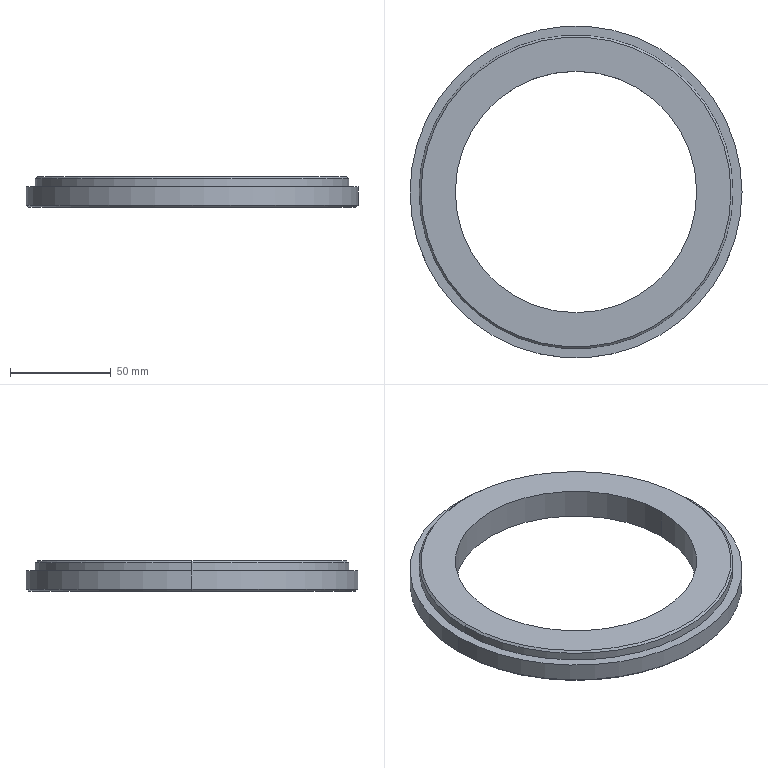Part | SolidWorks | features 3DProfileFeature 1, Chamfer 1, Extrusion 1, HoleWzd 1, ICE 1 | 1 solid | 37 faces | box 165 x 165 x 15 mm | volume 136481 mm3 | cylinder 18 | cone 16 | plane 3 | commonest cylinder face diameters 6.8 x12 120 x2 156 x2 165 x2
STEP:
#1=CARTESIAN_POINT('',(38.4,60.622,12.));
#2=VERTEX_POINT('',#1);
#3=CARTESIAN_POINT('',(31.6,60.622,12.));
#4=VERTEX_POINT('',#3);
#5=CARTESIAN_POINT('',(35.,60.622,12.));
#6=DIRECTION('',(0.,0.,-1.));
#7=DIRECTION('',(-1.,0.,0.));
#8=AXIS2_PLACEMENT_3D('',#5,#6,#7);
#9=CIRCLE('',#8,3.4);
#10=EDGE_CURVE('',#2,#4,#9,.T.);
#11=ORIENTED_EDGE('',*,*,#10,.F.);
#12=CARTESIAN_POINT('',(38.4,60.622,0.));
#13=VERTEX_POINT('',#12);
#14=CARTESIAN_POINT('',(38.4,60.622,0.));
#15=DIRECTION('',(0.,0.,-1.));
#16=VECTOR('',#15,1000.);
#17=LINE('',#14,#16);
#18=EDGE_CURVE('',#2,#13,#17,.T.);
#19=ORIENTED_EDGE('',*,*,#18,.T.);
#20=CARTESIAN_POINT('',(31.6,60.622,0.));
#21=VERTEX_POINT('',#20);
#22=CARTESIAN_POINT('',(35.,60.622,0.));
#23=DIRECTION('',(0.,0.,-1.));
#24=DIRECTION('',(-1.,0.,0.));
#25=AXIS2_PLACEMENT_3D('',#22,#23,#24);
#26=CIRCLE('',#25,3.4);
#27=EDGE_CURVE('',#13,#21,#26,.T.);
#28=ORIENTED_EDGE('',*,*,#27,.T.);
#29=CARTESIAN_POINT('',(31.6,60.622,0.));
#30=DIRECTION('',(0.,0.,-1.));
#31=VECTOR('',#30,1000.);
#32=LINE('',#29,#31);
#33=EDGE_CURVE('',#4,#21,#32,.T.);
#34=ORIENTED_EDGE('',*,*,#33,.F.);
#35=EDGE_LOOP('',(#11,#19,#28,#34));
#36=FACE_OUTER_BOUND('',#35,.T.);
#37=CARTESIAN_POINT('',(35.,60.622,0.));
#38=DIRECTION('',(0.,0.,-1.));
#39=DIRECTION('',(-1.,0.,0.));
#40=AXIS2_PLACEMENT_3D('',#37,#38,#39);
#41=CYLINDRICAL_SURFACE('',#40,3.4);
#42=ADVANCED_FACE('',(#36),#41,.F.);
#43=CARTESIAN_POINT('',(35.,60.622,14.043));
#44=VERTEX_POINT('',#43);
#45=CARTESIAN_POINT('',(31.6,60.622,12.));
#46=DIRECTION('',(-0.8572,0.,-0.515));
#47=VECTOR('',#46,1000.);
#48=LINE('',#45,#47);
#49=EDGE_CURVE('',#44,#4,#48,.T.);
#50=ORIENTED_EDGE('',*,*,#49,.F.);
#51=CARTESIAN_POINT('',(38.4,60.622,12.));
#52=DIRECTION('',(0.8572,0.,-0.515));
#53=VECTOR('',#52,1000.);
#54=LINE('',#51,#53);
#55=EDGE_CURVE('',#44,#2,#54,.T.);
#56=ORIENTED_EDGE('',*,*,#55,.T.);
#57=ORIENTED_EDGE('',*,*,#10,.T.);
#58=EDGE_LOOP('',(#50,#56,#57));
#59=FACE_OUTER_BOUND('',#58,.T.);
#60=CARTESIAN_POINT('',(35.,60.622,12.));
#61=DIRECTION('',(0.,0.,-1.));
#62=DIRECTION('',(-1.,0.,0.));
#63=AXIS2_PLACEMENT_3D('',#60,#61,#62);
#64=CONICAL_SURFACE('',#63,3.4,1.03);
#65=ADVANCED_FACE('',(#59),#64,.F.);
#66=CARTESIAN_POINT('',(-31.6,60.622,12.));
#67=VERTEX_POINT('',#66);
#68=CARTESIAN_POINT('',(-38.4,60.622,12.));
#69=VERTEX_POINT('',#68);
#70=CARTESIAN_POINT('',(-35.,60.622,12.));
#71=DIRECTION('',(0.,0.,-1.));
#72=DIRECTION('',(-1.,0.,0.));
#73=AXIS2_PLACEMENT_3D('',#70,#71,#72);
#74=CIRCLE('',#73,3.4);
#75=EDGE_CURVE('',#67,#69,#74,.T.);
#76=ORIENTED_EDGE('',*,*,#75,.F.);
#77=CARTESIAN_POINT('',(-31.6,60.622,0.));
#78=VERTEX_POINT('',#77);
#79=CARTESIAN_POINT('',(-31.6,60.622,0.));
#80=DIRECTION('',(0.,0.,-1.));
#81=VECTOR('',#80,1000.);
#82=LINE('',#79,#81);
#83=EDGE_CURVE('',#67,#78,#82,.T.);
#84=ORIENTED_EDGE('',*,*,#83,.T.);
#85=CARTESIAN_POINT('',(-38.4,60.622,0.));
#86=VERTEX_POINT('',#85);
#87=CARTESIAN_POINT('',(-35.,60.622,0.));
#88=DIRECTION('',(0.,0.,-1.));
#89=DIRECTION('',(-1.,0.,0.));
#90=AXIS2_PLACEMENT_3D('',#87,#88,#89);
#91=CIRCLE('',#90,3.4);
#92=EDGE_CURVE('',#78,#86,#91,.T.);
#93=ORIENTED_EDGE('',*,*,#92,.T.);
#94=CARTESIAN_POINT('',(-38.4,60.622,0.));
#95=DIRECTION('',(0.,0.,-1.));
#96=VECTOR('',#95,1000.);
#97=LINE('',#94,#96);
#98=EDGE_CURVE('',#69,#86,#97,.T.);
#99=ORIENTED_EDGE('',*,*,#98,.F.);
#100=EDGE_LOOP('',(#76,#84,#93,#99));
#101=FACE_OUTER_BOUND('',#100,.T.);
#102=CARTESIAN_POINT('',(-35.,60.622,0.));
#103=DIRECTION('',(0.,0.,-1.));
#104=DIRECTION('',(-1.,0.,0.));
#105=AXIS2_PLACEMENT_3D('',#102,#103,#104);
#106=CYLINDRICAL_SURFACE('',#105,3.4);
#107=ADVANCED_FACE('',(#101),#106,.F.);
#108=CARTESIAN_POINT('',(-35.,60.622,14.043));
#109=VERTEX_POINT('',#108);
#110=CARTESIAN_POINT('',(-38.4,60.622,12.));
#111=DIRECTION('',(-0.8572,0.,-0.515));
#112=VECTOR('',#111,1000.);
#113=LINE('',#110,#112);
#114=EDGE_CURVE('',#109,#69,#113,.T.);
#115=ORIENTED_EDGE('',*,*,#114,.F.);
#116=CARTESIAN_POINT('',(-31.6,60.622,12.));
#117=DIRECTION('',(0.8572,0.,-0.515));
#118=VECTOR('',#117,1000.);
#119=LINE('',#116,#118);
#120=EDGE_CURVE('',#109,#67,#119,.T.);
#121=ORIENTED_EDGE('',*,*,#120,.T.);
#122=ORIENTED_EDGE('',*,*,#75,.T.);
#123=EDGE_LOOP('',(#115,#121,#122));
#124=FACE_OUTER_BOUND('',#123,.T.);
#125=CARTESIAN_POINT('',(-35.,60.622,12.));
#126=DIRECTION('',(0.,0.,-1.));
#127=DIRECTION('',(-1.,0.,0.));
#128=AXIS2_PLACEMENT_3D('',#125,#126,#127);
#129=CONICAL_SURFACE('',#128,3.4,1.03);
#130=ADVANCED_FACE('',(#124),#129,.F.);
#131=CARTESIAN_POINT('',(-66.6,0.,12.));
#132=VERTEX_POINT('',#131);
#133=CARTESIAN_POINT('',(-73.4,0.,12.));
#134=VERTEX_POINT('',#133);
#135=CARTESIAN_POINT('',(-70.,0.,12.));
#136=DIRECTION('',(0.,0.,-1.));
#137=DIRECTION('',(-1.,0.,0.));
#138=AXIS2_PLACEMENT_3D('',#135,#136,#137);
#139=CIRCLE('',#138,3.4);
#140=EDGE_CURVE('',#132,#134,#139,.T.);
#141=ORIENTED_EDGE('',*,*,#140,.F.);
#142=CARTESIAN_POINT('',(-66.6,0.,0.));
#143=VERTEX_POINT('',#142);
#144=CARTESIAN_POINT('',(-66.6,0.,0.));
#145=DIRECTION('',(0.,0.,-1.));
#146=VECTOR('',#145,1000.);
#147=LINE('',#144,#146);
#148=EDGE_CURVE('',#132,#143,#147,.T.);
#149=ORIENTED_EDGE('',*,*,#148,.T.);
#150=CARTESIAN_POINT('',(-73.4,0.,0.));
#151=VERTEX_POINT('',#150);
#152=CARTESIAN_POINT('',(-70.,0.,0.));
#153=DIRECTION('',(0.,0.,-1.));
#154=DIRECTION('',(-1.,0.,0.));
#155=AXIS2_PLACEMENT_3D('',#152,#153,#154);
#156=CIRCLE('',#155,3.4);
#157=EDGE_CURVE('',#143,#151,#156,.T.);
#158=ORIENTED_EDGE('',*,*,#157,.T.);
#159=CARTESIAN_POINT('',(-73.4,0.,0.));
#160=DIRECTION('',(0.,0.,-1.));
#161=VECTOR('',#160,1000.);
#162=LINE('',#159,#161);
#163=EDGE_CURVE('',#134,#151,#162,.T.);
#164=ORIENTED_EDGE('',*,*,#163,.F.);
#165=EDGE_LOOP('',(#141,#149,#158,#164));
#166=FACE_OUTER_BOUND('',#165,.T.);
#167=CARTESIAN_POINT('',(-70.,0.,0.));
#168=DIRECTION('',(0.,0.,-1.));
#169=DIRECTION('',(-1.,0.,0.));
#170=AXIS2_PLACEMENT_3D('',#167,#168,#169);
#171=CYLINDRICAL_SURFACE('',#170,3.4);
#172=ADVANCED_FACE('',(#166),#171,.F.);
#173=CARTESIAN_POINT('',(-70.,0.,14.043));
#174=VERTEX_POINT('',#173);
#175=CARTESIAN_POINT('',(-73.4,0.,12.));
#176=DIRECTION('',(-0.8572,0.,-0.515));
#177=VECTOR('',#176,1000.);
#178=LINE('',#175,#177);
#179=EDGE_CURVE('',#174,#134,#178,.T.);
#180=ORIENTED_EDGE('',*,*,#179,.F.);
#181=CARTESIAN_POINT('',(-66.6,0.,12.));
#182=DIRECTION('',(0.8572,0.,-0.515));
#183=VECTOR('',#182,1000.);
#184=LINE('',#181,#183);
#185=EDGE_CURVE('',#174,#132,#184,.T.);
#186=ORIENTED_EDGE('',*,*,#185,.T.);
#187=ORIENTED_EDGE('',*,*,#140,.T.);
#188=EDGE_LOOP('',(#180,#186,#187));
#189=FACE_OUTER_BOUND('',#188,.T.);
#190=CARTESIAN_POINT('',(-70.,0.,12.));
#191=DIRECTION('',(0.,0.,-1.));
#192=DIRECTION('',(-1.,0.,0.));
#193=AXIS2_PLACEMENT_3D('',#190,#191,#192);
#194=CONICAL_SURFACE('',#193,3.4,1.03);
#195=ADVANCED_FACE('',(#189),#194,.F.);
#196=CARTESIAN_POINT('',(-31.6,-60.622,12.));
#197=VERTEX_POINT('',#196);
#198=CARTESIAN_POINT('',(-38.4,-60.622,12.));
#199=VERTEX_POINT('',#198);
#200=CARTESIAN_POINT('',(-35.,-60.622,12.));
#201=DIRECTION('',(0.,0.,-1.));
#202=DIRECTION('',(-1.,0.,0.));
#203=AXIS2_PLACEMENT_3D('',#200,#201,#202);
#204=CIRCLE('',#203,3.4);
#205=EDGE_CURVE('',#197,#199,#204,.T.);
#206=ORIENTED_EDGE('',*,*,#205,.F.);
#207=CARTESIAN_POINT('',(-31.6,-60.622,0.));
#208=VERTEX_POINT('',#207);
#209=CARTESIAN_POINT('',(-31.6,-60.622,0.));
#210=DIRECTION('',(0.,0.,-1.));
#211=VECTOR('',#210,1000.);
#212=LINE('',#209,#211);
#213=EDGE_CURVE('',#197,#208,#212,.T.);
#214=ORIENTED_EDGE('',*,*,#213,.T.);
#215=CARTESIAN_POINT('',(-38.4,-60.622,0.));
#216=VERTEX_POINT('',#215);
#217=CARTESIAN_POINT('',(-35.,-60.622,0.));
#218=DIRECTION('',(0.,0.,-1.));
#219=DIRECTION('',(-1.,0.,0.));
#220=AXIS2_PLACEMENT_3D('',#217,#218,#219);
#221=CIRCLE('',#220,3.4);
#222=EDGE_CURVE('',#208,#216,#221,.T.);
#223=ORIENTED_EDGE('',*,*,#222,.T.);
#224=CARTESIAN_POINT('',(-38.4,-60.622,0.));
#225=DIRECTION('',(0.,0.,-1.));
#226=VECTOR('',#225,1000.);
#227=LINE('',#224,#226);
#228=EDGE_CURVE('',#199,#216,#227,.T.);
#229=ORIENTED_EDGE('',*,*,#228,.F.);
#230=EDGE_LOOP('',(#206,#214,#223,#229));
#231=FACE_OUTER_BOUND('',#230,.T.);
#232=CARTESIAN_POINT('',(-35.,-60.622,0.));
#233=DIRECTION('',(0.,0.,-1.));
#234=DIRECTION('',(-1.,0.,0.));
#235=AXIS2_PLACEMENT_3D('',#232,#233,#234);
#236=CYLINDRICAL_SURFACE('',#235,3.4);
#237=ADVANCED_FACE('',(#231),#236,.F.);
#238=CARTESIAN_POINT('',(-35.,-60.622,14.043));
#239=VERTEX_POINT('',#238);
#240=CARTESIAN_POINT('',(-38.4,-60.622,12.));
#241=DIRECTION('',(-0.8572,0.,-0.515));
#242=VECTOR('',#241,1000.);
#243=LINE('',#240,#242);
#244=EDGE_CURVE('',#239,#199,#243,.T.);
#245=ORIENTED_EDGE('',*,*,#244,.F.);
#246=CARTESIAN_POINT('',(-31.6,-60.622,12.));
#247=DIRECTION('',(0.8572,0.,-0.515));
#248=VECTOR('',#247,1000.);
#249=LINE('',#246,#248);
#250=EDGE_CURVE('',#239,#197,#249,.T.);
#251=ORIENTED_EDGE('',*,*,#250,.T.);
#252=ORIENTED_EDGE('',*,*,#205,.T.);
#253=EDGE_LOOP('',(#245,#251,#252));
#254=FACE_OUTER_BOUND('',#253,.T.);
#255=CARTESIAN_POINT('',(-35.,-60.622,12.));
#256=DIRECTION('',(0.,0.,-1.));
#257=DIRECTION('',(-1.,0.,0.));
#258=AXIS2_PLACEMENT_3D('',#255,#256,#257);
#259=CONICAL_SURFACE('',#258,3.4,1.03);
#260=ADVANCED_FACE('',(#254),#259,.F.);
#261=CARTESIAN_POINT('',(38.4,-60.622,12.));
#262=VERTEX_POINT('',#261);
#263=CARTESIAN_POINT('',(31.6,-60.622,12.));
#264=VERTEX_POINT('',#263);
#265=CARTESIAN_POINT('',(35.,-60.622,12.));
#266=DIRECTION('',(0.,0.,-1.));
#267=DIRECTION('',(-1.,0.,0.));
#268=AXIS2_PLACEMENT_3D('',#265,#266,#267);
#269=CIRCLE('',#268,3.4);
#270=EDGE_CURVE('',#262,#264,#269,.T.);
#271=ORIENTED_EDGE('',*,*,#270,.F.);
#272=CARTESIAN_POINT('',(38.4,-60.622,0.));
#273=VERTEX_POINT('',#272);
#274=CARTESIAN_POINT('',(38.4,-60.622,0.));
#275=DIRECTION('',(0.,0.,-1.));
#276=VECTOR('',#275,1000.);
#277=LINE('',#274,#276);
#278=EDGE_CURVE('',#262,#273,#277,.T.);
#279=ORIENTED_EDGE('',*,*,#278,.T.);
#280=CARTESIAN_POINT('',(31.6,-60.622,0.));
#281=VERTEX_POINT('',#280);
#282=CARTESIAN_POINT('',(35.,-60.622,0.));
#283=DIRECTION('',(0.,0.,-1.));
#284=DIRECTION('',(-1.,0.,0.));
#285=AXIS2_PLACEMENT_3D('',#282,#283,#284);
#286=CIRCLE('',#285,3.4);
#287=EDGE_CURVE('',#273,#281,#286,.T.);
#288=ORIENTED_EDGE('',*,*,#287,.T.);
#289=CARTESIAN_POINT('',(31.6,-60.622,0.));
#290=DIRECTION('',(0.,0.,-1.));
#291=VECTOR('',#290,1000.);
#292=LINE('',#289,#291);
#293=EDGE_CURVE('',#264,#281,#292,.T.);
#294=ORIENTED_EDGE('',*,*,#293,.F.);
#295=EDGE_LOOP('',(#271,#279,#288,#294));
#296=FACE_OUTER_BOUND('',#295,.T.);
#297=CARTESIAN_POINT('',(35.,-60.622,0.));
#298=DIRECTION('',(0.,0.,-1.));
#299=DIRECTION('',(-1.,0.,0.));
#300=AXIS2_PLACEMENT_3D('',#297,#298,#299);
#301=CYLINDRICAL_SURFACE('',#300,3.4);
#302=ADVANCED_FACE('',(#296),#301,.F.);
#303=CARTESIAN_POINT('',(35.,-60.622,14.043));
#304=VERTEX_POINT('',#303);
#305=CARTESIAN_POINT('',(31.6,-60.622,12.));
#306=DIRECTION('',(-0.8572,0.,-0.515));
#307=VECTOR('',#306,1000.);
#308=LINE('',#305,#307);
#309=EDGE_CURVE('',#304,#264,#308,.T.);
#310=ORIENTED_EDGE('',*,*,#309,.F.);
#311=CARTESIAN_POINT('',(38.4,-60.622,12.));
#312=DIRECTION('',(0.8572,0.,-0.515));
#313=VECTOR('',#312,1000.);
#314=LINE('',#311,#313);
#315=EDGE_CURVE('',#304,#262,#314,.T.);
#316=ORIENTED_EDGE('',*,*,#315,.T.);
#317=ORIENTED_EDGE('',*,*,#270,.T.);
#318=EDGE_LOOP('',(#310,#316,#317));
#319=FACE_OUTER_BOUND('',#318,.T.);
#320=CARTESIAN_POINT('',(35.,-60.622,12.));
#321=DIRECTION('',(0.,0.,-1.));
#322=DIRECTION('',(-1.,0.,0.));
#323=AXIS2_PLACEMENT_3D('',#320,#321,#322);
#324=CONICAL_SURFACE('',#323,3.4,1.03);
#325=ADVANCED_FACE('',(#319),#324,.F.);
#326=CARTESIAN_POINT('',(73.4,0.,12.));
#327=VERTEX_POINT('',#326);
#328=CARTESIAN_POINT('',(66.6,0.,12.));
#329=VERTEX_POINT('',#328);
#330=CARTESIAN_POINT('',(70.,0.,12.));
#331=DIRECTION('',(0.,0.,-1.));
#332=DIRECTION('',(-1.,0.,0.));
#333=AXIS2_PLACEMENT_3D('',#330,#331,#332);
#334=CIRCLE('',#333,3.4);
#335=EDGE_CURVE('',#327,#329,#334,.T.);
#336=ORIENTED_EDGE('',*,*,#335,.F.);
#337=CARTESIAN_POINT('',(73.4,0.,0.));
#338=VERTEX_POINT('',#337);
#339=CARTESIAN_POINT('',(73.4,0.,0.));
#340=DIRECTION('',(0.,0.,-1.));
#341=VECTOR('',#340,1000.);
#342=LINE('',#339,#341);
#343=EDGE_CURVE('',#327,#338,#342,.T.);
#344=ORIENTED_EDGE('',*,*,#343,.T.);
#345=CARTESIAN_POINT('',(66.6,0.,0.));
#346=VERTEX_POINT('',#345);
#347=CARTESIAN_POINT('',(70.,0.,0.));
#348=DIRECTION('',(0.,0.,-1.));
#349=DIRECTION('',(-1.,0.,0.));
#350=AXIS2_PLACEMENT_3D('',#347,#348,#349);
#351=CIRCLE('',#350,3.4);
#352=EDGE_CURVE('',#338,#346,#351,.T.);
#353=ORIENTED_EDGE('',*,*,#352,.T.);
#354=CARTESIAN_POINT('',(66.6,0.,0.));
#355=DIRECTION('',(0.,0.,-1.));
#356=VECTOR('',#355,1000.);
#357=LINE('',#354,#356);
#358=EDGE_CURVE('',#329,#346,#357,.T.);
#359=ORIENTED_EDGE('',*,*,#358,.F.);
#360=EDGE_LOOP('',(#336,#344,#353,#359));
#361=FACE_OUTER_BOUND('',#360,.T.);
#362=CARTESIAN_POINT('',(70.,0.,0.));
#363=DIRECTION('',(0.,0.,-1.));
#364=DIRECTION('',(-1.,0.,0.));
#365=AXIS2_PLACEMENT_3D('',#362,#363,#364);
#366=CYLINDRICAL_SURFACE('',#365,3.4);
#367=ADVANCED_FACE('',(#361),#366,.F.);
#368=CARTESIAN_POINT('',(70.,0.,14.043));
#369=VERTEX_POINT('',#368);
#370=CARTESIAN_POINT('',(66.6,0.,12.));
#371=DIRECTION('',(-0.8572,0.,-0.515));
#372=VECTOR('',#371,1000.);
#373=LINE('',#370,#372);
#374=EDGE_CURVE('',#369,#329,#373,.T.);
#375=ORIENTED_EDGE('',*,*,#374,.F.);
#376=CARTESIAN_POINT('',(73.4,0.,12.));
#377=DIRECTION('',(0.8572,0.,-0.515));
#378=VECTOR('',#377,1000.);
#379=LINE('',#376,#378);
#380=EDGE_CURVE('',#369,#327,#379,.T.);
#381=ORIENTED_EDGE('',*,*,#380,.T.);
#382=ORIENTED_EDGE('',*,*,#335,.T.);
#383=EDGE_LOOP('',(#375,#381,#382));
#384=FACE_OUTER_BOUND('',#383,.T.);
#385=CARTESIAN_POINT('',(70.,0.,12.));
#386=DIRECTION('',(0.,0.,-1.));
#387=DIRECTION('',(-1.,0.,0.));
#388=AXIS2_PLACEMENT_3D('',#385,#386,#387);
#389=CONICAL_SURFACE('',#388,3.4,1.03);
#390=ADVANCED_FACE('',(#384),#389,.F.);
#391=CARTESIAN_POINT('',(77.,0.,15.));
#392=VERTEX_POINT('',#391);
#393=CARTESIAN_POINT('',(-77.,0.,15.));
#394=VERTEX_POINT('',#393);
#395=CARTESIAN_POINT('',(0.,0.,15.));
#396=DIRECTION('',(0.,0.,1.));
#397=DIRECTION('',(1.,0.,0.));
#398=AXIS2_PLACEMENT_3D('',#395,#396,#397);
#399=CIRCLE('',#398,77.);
#400=EDGE_CURVE('',#392,#394,#399,.T.);
#401=ORIENTED_EDGE('',*,*,#400,.F.);
#402=CARTESIAN_POINT('',(78.,0.,14.));
#403=VERTEX_POINT('',#402);
#404=CARTESIAN_POINT('',(77.,0.,15.));
#405=DIRECTION('',(0.7071,0.,-0.7071));
#406=VECTOR('',#405,1000.);
#407=LINE('',#404,#406);
#408=EDGE_CURVE('',#392,#403,#407,.T.);
#409=ORIENTED_EDGE('',*,*,#408,.T.);
#410=CARTESIAN_POINT('',(-78.,0.,14.));
#411=VERTEX_POINT('',#410);
#412=CARTESIAN_POINT('',(0.,0.,14.));
#413=DIRECTION('',(0.,0.,-1.));
#414=DIRECTION('',(1.,0.,0.));
#415=AXIS2_PLACEMENT_3D('',#412,#413,#414);
#416=CIRCLE('',#415,78.);
#417=EDGE_CURVE('',#411,#403,#416,.T.);
#418=ORIENTED_EDGE('',*,*,#417,.F.);
#419=CARTESIAN_POINT('',(-77.,0.,15.));
#420=DIRECTION('',(-0.7071,0.,-0.7071));
#421=VECTOR('',#420,1000.);
#422=LINE('',#419,#421);
#423=EDGE_CURVE('',#394,#411,#422,.T.);
#424=ORIENTED_EDGE('',*,*,#423,.F.);
#425=EDGE_LOOP('',(#401,#409,#418,#424));
#426=FACE_OUTER_BOUND('',#425,.T.);
#427=CARTESIAN_POINT('',(0.,0.,15.));
#428=DIRECTION('',(0.,0.,-1.));
#429=DIRECTION('',(-1.,0.,0.));
#430=AXIS2_PLACEMENT_3D('',#427,#428,#429);
#431=CONICAL_SURFACE('',#430,77.,0.7854);
#432=ADVANCED_FACE('',(#426),#431,.T.);
#433=CARTESIAN_POINT('',(-81.5,0.,0.));
#434=VERTEX_POINT('',#433);
#435=CARTESIAN_POINT('',(81.5,0.,0.));
#436=VERTEX_POINT('',#435);
#437=CARTESIAN_POINT('',(0.,0.,0.));
#438=DIRECTION('',(0.,0.,-1.));
#439=DIRECTION('',(1.,0.,0.));
#440=AXIS2_PLACEMENT_3D('',#437,#438,#439);
#441=CIRCLE('',#440,81.5);
#442=EDGE_CURVE('',#434,#436,#441,.T.);
#443=ORIENTED_EDGE('',*,*,#442,.F.);
#444=CARTESIAN_POINT('',(-82.5,0.,1.));
#445=VERTEX_POINT('',#444);
#446=CARTESIAN_POINT('',(-82.5,0.,1.));
#447=DIRECTION('',(-0.7071,0.,0.7071));
#448=VECTOR('',#447,1000.);
#449=LINE('',#446,#448);
#450=EDGE_CURVE('',#434,#445,#449,.T.);
#451=ORIENTED_EDGE('',*,*,#450,.T.);
#452=CARTESIAN_POINT('',(82.5,0.,1.));
#453=VERTEX_POINT('',#452);
#454=CARTESIAN_POINT('',(0.,0.,1.));
#455=DIRECTION('',(0.,0.,1.));
#456=DIRECTION('',(1.,0.,0.));
#457=AXIS2_PLACEMENT_3D('',#454,#455,#456);
#458=CIRCLE('',#457,82.5);
#459=EDGE_CURVE('',#453,#445,#458,.T.);
#460=ORIENTED_EDGE('',*,*,#459,.F.);
#461=CARTESIAN_POINT('',(82.5,0.,1.));
#462=DIRECTION('',(0.7071,0.,0.7071));
#463=VECTOR('',#462,1000.);
#464=LINE('',#461,#463);
#465=EDGE_CURVE('',#436,#453,#464,.T.);
#466=ORIENTED_EDGE('',*,*,#465,.F.);
#467=EDGE_LOOP('',(#443,#451,#460,#466));
#468=FACE_OUTER_BOUND('',#467,.T.);
#469=CARTESIAN_POINT('',(0.,0.,1.));
#470=DIRECTION('',(0.,0.,1.));
#471=DIRECTION('',(1.,0.,0.));
#472=AXIS2_PLACEMENT_3D('',#469,#470,#471);
#473=CONICAL_SURFACE('',#472,82.5,0.7854);
#474=ADVANCED_FACE('',(#468),#473,.T.);
#475=ORIENTED_EDGE('',*,*,#417,.T.);
#476=CARTESIAN_POINT('',(78.,0.,10.));
#477=VERTEX_POINT('',#476);
#478=CARTESIAN_POINT('',(78.,0.,15.));
#479=DIRECTION('',(0.,0.,-1.));
#480=VECTOR('',#479,1000.);
#481=LINE('',#478,#480);
#482=EDGE_CURVE('',#403,#477,#481,.T.);
#483=ORIENTED_EDGE('',*,*,#482,.T.);
#484=CARTESIAN_POINT('',(-78.,0.,10.));
#485=VERTEX_POINT('',#484);
#486=CARTESIAN_POINT('',(0.,0.,10.));
#487=DIRECTION('',(0.,0.,1.));
#488=DIRECTION('',(1.,0.,0.));
#489=AXIS2_PLACEMENT_3D('',#486,#487,#488);
#490=CIRCLE('',#489,78.);
#491=EDGE_CURVE('',#477,#485,#490,.T.);
#492=ORIENTED_EDGE('',*,*,#491,.T.);
#493=CARTESIAN_POINT('',(-78.,0.,15.));
#494=DIRECTION('',(0.,0.,-1.));
#495=VECTOR('',#494,1000.);
#496=LINE('',#493,#495);
#497=EDGE_CURVE('',#411,#485,#496,.T.);
#498=ORIENTED_EDGE('',*,*,#497,.F.);
#499=EDGE_LOOP('',(#475,#483,#492,#498));
#500=FACE_OUTER_BOUND('',#499,.T.);
#501=CARTESIAN_POINT('',(0.,0.,15.));
#502=DIRECTION('',(0.,0.,-1.));
#503=DIRECTION('',(-1.,0.,0.));
#504=AXIS2_PLACEMENT_3D('',#501,#502,#503);
#505=CYLINDRICAL_SURFACE('',#504,78.);
#506=ADVANCED_FACE('',(#500),#505,.T.);
#507=CARTESIAN_POINT('',(-60.,0.,15.));
#508=VERTEX_POINT('',#507);
#509=CARTESIAN_POINT('',(60.,0.,15.));
#510=VERTEX_POINT('',#509);
#511=CARTESIAN_POINT('',(0.,0.,15.));
#512=DIRECTION('',(0.,0.,1.));
#513=DIRECTION('',(1.,0.,0.));
#514=AXIS2_PLACEMENT_3D('',#511,#512,#513);
#515=CIRCLE('',#514,60.);
#516=EDGE_CURVE('',#508,#510,#515,.T.);
#517=ORIENTED_EDGE('',*,*,#516,.T.);
#518=CARTESIAN_POINT('',(60.,0.,0.));
#519=VERTEX_POINT('',#518);
#520=CARTESIAN_POINT('',(60.,0.,10.));
#521=DIRECTION('',(0.,0.,-1.));
#522=VECTOR('',#521,1000.);
#523=LINE('',#520,#522);
#524=EDGE_CURVE('',#510,#519,#523,.T.);
#525=ORIENTED_EDGE('',*,*,#524,.T.);
#526=CARTESIAN_POINT('',(-60.,0.,0.));
#527=VERTEX_POINT('',#526);
#528=CARTESIAN_POINT('',(0.,0.,0.));
#529=DIRECTION('',(0.,0.,1.));
#530=DIRECTION('',(1.,0.,0.));
#531=AXIS2_PLACEMENT_3D('',#528,#529,#530);
#532=CIRCLE('',#531,60.);
#533=EDGE_CURVE('',#527,#519,#532,.T.);
#534=ORIENTED_EDGE('',*,*,#533,.F.);
#535=CARTESIAN_POINT('',(-60.,0.,10.));
#536=DIRECTION('',(0.,0.,-1.));
#537=VECTOR('',#536,1000.);
#538=LINE('',#535,#537);
#539=EDGE_CURVE('',#508,#527,#538,.T.);
#540=ORIENTED_EDGE('',*,*,#539,.F.);
#541=EDGE_LOOP('',(#517,#525,#534,#540));
#542=FACE_OUTER_BOUND('',#541,.T.);
#543=CARTESIAN_POINT('',(0.,0.,10.));
#544=DIRECTION('',(0.,0.,-1.));
#545=DIRECTION('',(-1.,0.,0.));
#546=AXIS2_PLACEMENT_3D('',#543,#544,#545);
#547=CYLINDRICAL_SURFACE('',#546,60.);
#548=ADVANCED_FACE('',(#542),#547,.F.);
#549=CARTESIAN_POINT('',(82.5,0.,10.));
#550=VERTEX_POINT('',#549);
#551=CARTESIAN_POINT('',(-82.5,0.,10.));
#552=VERTEX_POINT('',#551);
#553=CARTESIAN_POINT('',(0.,0.,10.));
#554=DIRECTION('',(0.,0.,1.));
#555=DIRECTION('',(1.,0.,0.));
#556=AXIS2_PLACEMENT_3D('',#553,#554,#555);
#557=CIRCLE('',#556,82.5);
#558=EDGE_CURVE('',#550,#552,#557,.T.);
#559=ORIENTED_EDGE('',*,*,#558,.F.);
#560=CARTESIAN_POINT('',(82.5,0.,10.));
#561=DIRECTION('',(0.,0.,-1.));
#562=VECTOR('',#561,1000.);
#563=LINE('',#560,#562);
#564=EDGE_CURVE('',#550,#453,#563,.T.);
#565=ORIENTED_EDGE('',*,*,#564,.T.);
#566=ORIENTED_EDGE('',*,*,#459,.T.);
#567=CARTESIAN_POINT('',(-82.5,0.,10.));
#568=DIRECTION('',(0.,0.,-1.));
#569=VECTOR('',#568,1000.);
#570=LINE('',#567,#569);
#571=EDGE_CURVE('',#552,#445,#570,.T.);
#572=ORIENTED_EDGE('',*,*,#571,.F.);
#573=EDGE_LOOP('',(#559,#565,#566,#572));
#574=FACE_OUTER_BOUND('',#573,.T.);
#575=CARTESIAN_POINT('',(0.,0.,10.));
#576=DIRECTION('',(0.,0.,-1.));
#577=DIRECTION('',(-1.,0.,0.));
#578=AXIS2_PLACEMENT_3D('',#575,#576,#577);
#579=CYLINDRICAL_SURFACE('',#578,82.5);
#580=ADVANCED_FACE('',(#574),#579,.T.);
#581=CARTESIAN_POINT('',(0.,0.,10.));
#582=DIRECTION('',(0.,0.,1.));
#583=DIRECTION('',(1.,0.,0.));
#584=AXIS2_PLACEMENT_3D('',#581,#582,#583);
#585=CIRCLE('',#584,82.5);
#586=EDGE_CURVE('',#552,#550,#585,.T.);
#587=ORIENTED_EDGE('',*,*,#586,.T.);
#588=ORIENTED_EDGE('',*,*,#558,.T.);
#589=EDGE_LOOP('',(#587,#588));
#590=FACE_OUTER_BOUND('',#589,.T.);
#591=CARTESIAN_POINT('',(0.,0.,10.));
#592=DIRECTION('',(0.,0.,1.));
#593=DIRECTION('',(1.,0.,0.));
#594=AXIS2_PLACEMENT_3D('',#591,#592,#593);
#595=CIRCLE('',#594,78.);
#596=EDGE_CURVE('',#485,#477,#595,.T.);
#597=ORIENTED_EDGE('',*,*,#596,.F.);
#598=ORIENTED_EDGE('',*,*,#491,.F.);
#599=EDGE_LOOP('',(#597,#598));
#600=FACE_BOUND('',#599,.T.);
#601=CARTESIAN_POINT('',(0.,0.,10.));
#602=DIRECTION('',(0.,0.,1.));
#603=DIRECTION('',(1.,0.,0.));
#604=AXIS2_PLACEMENT_3D('',#601,#602,#603);
#605=PLANE('',#604);
#606=ADVANCED_FACE('',(#590,#600),#605,.T.);
#607=CARTESIAN_POINT('',(35.,60.622,0.));
#608=DIRECTION('',(0.,0.,-1.));
#609=DIRECTION('',(-1.,0.,0.));
#610=AXIS2_PLACEMENT_3D('',#607,#608,#609);
#611=CIRCLE('',#610,3.4);
#612=EDGE_CURVE('',#21,#13,#611,.T.);
#613=ORIENTED_EDGE('',*,*,#612,.F.);
#614=ORIENTED_EDGE('',*,*,#27,.F.);
#615=EDGE_LOOP('',(#613,#614));
#616=FACE_BOUND('',#615,.T.);
#617=CARTESIAN_POINT('',(-35.,60.622,0.));
#618=DIRECTION('',(0.,0.,-1.));
#619=DIRECTION('',(-1.,0.,0.));
#620=AXIS2_PLACEMENT_3D('',#617,#618,#619);
#621=CIRCLE('',#620,3.4);
#622=EDGE_CURVE('',#86,#78,#621,.T.);
#623=ORIENTED_EDGE('',*,*,#622,.F.);
#624=ORIENTED_EDGE('',*,*,#92,.F.);
#625=EDGE_LOOP('',(#623,#624));
#626=FACE_BOUND('',#625,.T.);
#627=CARTESIAN_POINT('',(-70.,0.,0.));
#628=DIRECTION('',(0.,0.,-1.));
#629=DIRECTION('',(-1.,0.,0.));
#630=AXIS2_PLACEMENT_3D('',#627,#628,#629);
#631=CIRCLE('',#630,3.4);
#632=EDGE_CURVE('',#151,#143,#631,.T.);
#633=ORIENTED_EDGE('',*,*,#632,.F.);
#634=ORIENTED_EDGE('',*,*,#157,.F.);
#635=EDGE_LOOP('',(#633,#634));
#636=FACE_BOUND('',#635,.T.);
#637=CARTESIAN_POINT('',(-35.,-60.622,0.));
#638=DIRECTION('',(0.,0.,-1.));
#639=DIRECTION('',(-1.,0.,0.));
#640=AXIS2_PLACEMENT_3D('',#637,#638,#639);
#641=CIRCLE('',#640,3.4);
#642=EDGE_CURVE('',#216,#208,#641,.T.);
#643=ORIENTED_EDGE('',*,*,#642,.F.);
#644=ORIENTED_EDGE('',*,*,#222,.F.);
#645=EDGE_LOOP('',(#643,#644));
#646=FACE_BOUND('',#645,.T.);
#647=CARTESIAN_POINT('',(35.,-60.622,0.));
#648=DIRECTION('',(0.,0.,-1.));
#649=DIRECTION('',(-1.,0.,0.));
#650=AXIS2_PLACEMENT_3D('',#647,#648,#649);
#651=CIRCLE('',#650,3.4);
#652=EDGE_CURVE('',#281,#273,#651,.T.);
#653=ORIENTED_EDGE('',*,*,#652,.F.);
#654=ORIENTED_EDGE('',*,*,#287,.F.);
#655=EDGE_LOOP('',(#653,#654));
#656=FACE_BOUND('',#655,.T.);
#657=CARTESIAN_POINT('',(70.,0.,0.));
#658=DIRECTION('',(0.,0.,-1.));
#659=DIRECTION('',(-1.,0.,0.));
#660=AXIS2_PLACEMENT_3D('',#657,#658,#659);
#661=CIRCLE('',#660,3.4);
#662=EDGE_CURVE('',#346,#338,#661,.T.);
#663=ORIENTED_EDGE('',*,*,#662,.F.);
#664=ORIENTED_EDGE('',*,*,#352,.F.);
#665=EDGE_LOOP('',(#663,#664));
#666=FACE_BOUND('',#665,.T.);
#667=CARTESIAN_POINT('',(0.,0.,0.));
#668=DIRECTION('',(0.,0.,-1.));
#669=DIRECTION('',(1.,0.,0.));
#670=AXIS2_PLACEMENT_3D('',#667,#668,#669);
#671=CIRCLE('',#670,81.5);
#672=EDGE_CURVE('',#436,#434,#671,.T.);
#673=ORIENTED_EDGE('',*,*,#672,.T.);
#674=ORIENTED_EDGE('',*,*,#442,.T.);
#675=EDGE_LOOP('',(#673,#674));
#676=FACE_OUTER_BOUND('',#675,.T.);
#677=ORIENTED_EDGE('',*,*,#533,.T.);
#678=CARTESIAN_POINT('',(0.,0.,0.));
#679=DIRECTION('',(0.,0.,1.));
#680=DIRECTION('',(1.,0.,0.));
#681=AXIS2_PLACEMENT_3D('',#678,#679,#680);
#682=CIRCLE('',#681,60.);
#683=EDGE_CURVE('',#519,#527,#682,.T.);
#684=ORIENTED_EDGE('',*,*,#683,.T.);
#685=EDGE_LOOP('',(#677,#684));
#686=FACE_BOUND('',#685,.T.);
#687=CARTESIAN_POINT('',(0.,0.,0.));
#688=DIRECTION('',(0.,0.,1.));
#689=DIRECTION('',(1.,0.,0.));
#690=AXIS2_PLACEMENT_3D('',#687,#688,#689);
#691=PLANE('',#690);
#692=ADVANCED_FACE('',(#616,#626,#636,#646,#656,#666,#676,#686),#691,.F.);
#693=ORIENTED_EDGE('',*,*,#564,.F.);
#694=ORIENTED_EDGE('',*,*,#586,.F.);
#695=ORIENTED_EDGE('',*,*,#571,.T.);
#696=CARTESIAN_POINT('',(0.,0.,1.));
#697=DIRECTION('',(0.,0.,1.));
#698=DIRECTION('',(1.,0.,0.));
#699=AXIS2_PLACEMENT_3D('',#696,#697,#698);
#700=CIRCLE('',#699,82.5);
#701=EDGE_CURVE('',#445,#453,#700,.T.);
#702=ORIENTED_EDGE('',*,*,#701,.T.);
#703=EDGE_LOOP('',(#693,#694,#695,#702));
#704=FACE_OUTER_BOUND('',#703,.T.);
#705=CARTESIAN_POINT('',(0.,0.,10.));
#706=DIRECTION('',(0.,0.,-1.));
#707=DIRECTION('',(-1.,0.,0.));
#708=AXIS2_PLACEMENT_3D('',#705,#706,#707);
#709=CYLINDRICAL_SURFACE('',#708,82.5);
#710=ADVANCED_FACE('',(#704),#709,.T.);
#711=ORIENTED_EDGE('',*,*,#524,.F.);
#712=CARTESIAN_POINT('',(0.,0.,15.));
#713=DIRECTION('',(0.,0.,1.));
#714=DIRECTION('',(1.,0.,0.));
#715=AXIS2_PLACEMENT_3D('',#712,#713,#714);
#716=CIRCLE('',#715,60.);
#717=EDGE_CURVE('',#510,#508,#716,.T.);
#718=ORIENTED_EDGE('',*,*,#717,.T.);
#719=ORIENTED_EDGE('',*,*,#539,.T.);
#720=ORIENTED_EDGE('',*,*,#683,.F.);
#721=EDGE_LOOP('',(#711,#718,#719,#720));
#722=FACE_OUTER_BOUND('',#721,.T.);
#723=CARTESIAN_POINT('',(0.,0.,10.));
#724=DIRECTION('',(0.,0.,-1.));
#725=DIRECTION('',(-1.,0.,0.));
#726=AXIS2_PLACEMENT_3D('',#723,#724,#725);
#727=CYLINDRICAL_SURFACE('',#726,60.);
#728=ADVANCED_FACE('',(#722),#727,.F.);
#729=CARTESIAN_POINT('',(0.,0.,15.));
#730=DIRECTION('',(0.,0.,1.));
#731=DIRECTION('',(1.,0.,0.));
#732=AXIS2_PLACEMENT_3D('',#729,#730,#731);
#733=CIRCLE('',#732,77.);
#734=EDGE_CURVE('',#394,#392,#733,.T.);
#735=ORIENTED_EDGE('',*,*,#734,.T.);
#736=ORIENTED_EDGE('',*,*,#400,.T.);
#737=EDGE_LOOP('',(#735,#736));
#738=FACE_OUTER_BOUND('',#737,.T.);
#739=ORIENTED_EDGE('',*,*,#516,.F.);
#740=ORIENTED_EDGE('',*,*,#717,.F.);
#741=EDGE_LOOP('',(#739,#740));
#742=FACE_BOUND('',#741,.T.);
#743=CARTESIAN_POINT('',(0.,0.,15.));
#744=DIRECTION('',(0.,0.,1.));
#745=DIRECTION('',(1.,0.,0.));
#746=AXIS2_PLACEMENT_3D('',#743,#744,#745);
#747=PLANE('',#746);
#748=ADVANCED_FACE('',(#738,#742),#747,.T.);
#749=ORIENTED_EDGE('',*,*,#482,.F.);
#750=CARTESIAN_POINT('',(0.,0.,14.));
#751=DIRECTION('',(0.,0.,-1.));
#752=DIRECTION('',(1.,0.,0.));
#753=AXIS2_PLACEMENT_3D('',#750,#751,#752);
#754=CIRCLE('',#753,78.);
#755=EDGE_CURVE('',#403,#411,#754,.T.);
#756=ORIENTED_EDGE('',*,*,#755,.T.);
#757=ORIENTED_EDGE('',*,*,#497,.T.);
#758=ORIENTED_EDGE('',*,*,#596,.T.);
#759=EDGE_LOOP('',(#749,#756,#757,#758));
#760=FACE_OUTER_BOUND('',#759,.T.);
#761=CARTESIAN_POINT('',(0.,0.,15.));
#762=DIRECTION('',(0.,0.,-1.));
#763=DIRECTION('',(-1.,0.,0.));
#764=AXIS2_PLACEMENT_3D('',#761,#762,#763);
#765=CYLINDRICAL_SURFACE('',#764,78.);
#766=ADVANCED_FACE('',(#760),#765,.T.);
#767=ORIENTED_EDGE('',*,*,#450,.F.);
#768=ORIENTED_EDGE('',*,*,#672,.F.);
#769=ORIENTED_EDGE('',*,*,#465,.T.);
#770=ORIENTED_EDGE('',*,*,#701,.F.);
#771=EDGE_LOOP('',(#767,#768,#769,#770));
#772=FACE_OUTER_BOUND('',#771,.T.);
#773=CARTESIAN_POINT('',(0.,0.,1.));
#774=DIRECTION('',(0.,0.,1.));
#775=DIRECTION('',(1.,0.,0.));
#776=AXIS2_PLACEMENT_3D('',#773,#774,#775);
#777=CONICAL_SURFACE('',#776,82.5,0.7854);
#778=ADVANCED_FACE('',(#772),#777,.T.);
#779=ORIENTED_EDGE('',*,*,#408,.F.);
#780=ORIENTED_EDGE('',*,*,#734,.F.);
#781=ORIENTED_EDGE('',*,*,#423,.T.);
#782=ORIENTED_EDGE('',*,*,#755,.F.);
#783=EDGE_LOOP('',(#779,#780,#781,#782));
#784=FACE_OUTER_BOUND('',#783,.T.);
#785=CARTESIAN_POINT('',(0.,0.,15.));
#786=DIRECTION('',(0.,0.,-1.));
#787=DIRECTION('',(-1.,0.,0.));
#788=AXIS2_PLACEMENT_3D('',#785,#786,#787);
#789=CONICAL_SURFACE('',#788,77.,0.7854);
#790=ADVANCED_FACE('',(#784),#789,.T.);
#791=ORIENTED_EDGE('',*,*,#380,.F.);
#792=ORIENTED_EDGE('',*,*,#374,.T.);
#793=CARTESIAN_POINT('',(70.,0.,12.));
#794=DIRECTION('',(0.,0.,-1.));
#795=DIRECTION('',(-1.,0.,0.));
#796=AXIS2_PLACEMENT_3D('',#793,#794,#795);
#797=CIRCLE('',#796,3.4);
#798=EDGE_CURVE('',#329,#327,#797,.T.);
#799=ORIENTED_EDGE('',*,*,#798,.T.);
#800=EDGE_LOOP('',(#791,#792,#799));
#801=FACE_OUTER_BOUND('',#800,.T.);
#802=CARTESIAN_POINT('',(70.,0.,12.));
#803=DIRECTION('',(0.,0.,-1.));
#804=DIRECTION('',(-1.,0.,0.));
#805=AXIS2_PLACEMENT_3D('',#802,#803,#804);
#806=CONICAL_SURFACE('',#805,3.4,1.03);
#807=ADVANCED_FACE('',(#801),#806,.F.);
#808=ORIENTED_EDGE('',*,*,#343,.F.);
#809=ORIENTED_EDGE('',*,*,#798,.F.);
#810=ORIENTED_EDGE('',*,*,#358,.T.);
#811=ORIENTED_EDGE('',*,*,#662,.T.);
#812=EDGE_LOOP('',(#808,#809,#810,#811));
#813=FACE_OUTER_BOUND('',#812,.T.);
#814=CARTESIAN_POINT('',(70.,0.,0.));
#815=DIRECTION('',(0.,0.,-1.));
#816=DIRECTION('',(-1.,0.,0.));
#817=AXIS2_PLACEMENT_3D('',#814,#815,#816);
#818=CYLINDRICAL_SURFACE('',#817,3.4);
#819=ADVANCED_FACE('',(#813),#818,.F.);
#820=ORIENTED_EDGE('',*,*,#315,.F.);
#821=ORIENTED_EDGE('',*,*,#309,.T.);
#822=CARTESIAN_POINT('',(35.,-60.622,12.));
#823=DIRECTION('',(0.,0.,-1.));
#824=DIRECTION('',(-1.,0.,0.));
#825=AXIS2_PLACEMENT_3D('',#822,#823,#824);
#826=CIRCLE('',#825,3.4);
#827=EDGE_CURVE('',#264,#262,#826,.T.);
#828=ORIENTED_EDGE('',*,*,#827,.T.);
#829=EDGE_LOOP('',(#820,#821,#828));
#830=FACE_OUTER_BOUND('',#829,.T.);
#831=CARTESIAN_POINT('',(35.,-60.622,12.));
#832=DIRECTION('',(0.,0.,-1.));
#833=DIRECTION('',(-1.,0.,0.));
#834=AXIS2_PLACEMENT_3D('',#831,#832,#833);
#835=CONICAL_SURFACE('',#834,3.4,1.03);
#836=ADVANCED_FACE('',(#830),#835,.F.);
#837=ORIENTED_EDGE('',*,*,#278,.F.);
#838=ORIENTED_EDGE('',*,*,#827,.F.);
#839=ORIENTED_EDGE('',*,*,#293,.T.);
#840=ORIENTED_EDGE('',*,*,#652,.T.);
#841=EDGE_LOOP('',(#837,#838,#839,#840));
#842=FACE_OUTER_BOUND('',#841,.T.);
#843=CARTESIAN_POINT('',(35.,-60.622,0.));
#844=DIRECTION('',(0.,0.,-1.));
#845=DIRECTION('',(-1.,0.,0.));
#846=AXIS2_PLACEMENT_3D('',#843,#844,#845);
#847=CYLINDRICAL_SURFACE('',#846,3.4);
#848=ADVANCED_FACE('',(#842),#847,.F.);
#849=ORIENTED_EDGE('',*,*,#250,.F.);
#850=ORIENTED_EDGE('',*,*,#244,.T.);
#851=CARTESIAN_POINT('',(-35.,-60.622,12.));
#852=DIRECTION('',(0.,0.,-1.));
#853=DIRECTION('',(-1.,0.,0.));
#854=AXIS2_PLACEMENT_3D('',#851,#852,#853);
#855=CIRCLE('',#854,3.4);
#856=EDGE_CURVE('',#199,#197,#855,.T.);
#857=ORIENTED_EDGE('',*,*,#856,.T.);
#858=EDGE_LOOP('',(#849,#850,#857));
#859=FACE_OUTER_BOUND('',#858,.T.);
#860=CARTESIAN_POINT('',(-35.,-60.622,12.));
#861=DIRECTION('',(0.,0.,-1.));
#862=DIRECTION('',(-1.,0.,0.));
#863=AXIS2_PLACEMENT_3D('',#860,#861,#862);
#864=CONICAL_SURFACE('',#863,3.4,1.03);
#865=ADVANCED_FACE('',(#859),#864,.F.);
#866=ORIENTED_EDGE('',*,*,#213,.F.);
#867=ORIENTED_EDGE('',*,*,#856,.F.);
#868=ORIENTED_EDGE('',*,*,#228,.T.);
#869=ORIENTED_EDGE('',*,*,#642,.T.);
#870=EDGE_LOOP('',(#866,#867,#868,#869));
#871=FACE_OUTER_BOUND('',#870,.T.);
#872=CARTESIAN_POINT('',(-35.,-60.622,0.));
#873=DIRECTION('',(0.,0.,-1.));
#874=DIRECTION('',(-1.,0.,0.));
#875=AXIS2_PLACEMENT_3D('',#872,#873,#874);
#876=CYLINDRICAL_SURFACE('',#875,3.4);
#877=ADVANCED_FACE('',(#871),#876,.F.);
#878=ORIENTED_EDGE('',*,*,#185,.F.);
#879=ORIENTED_EDGE('',*,*,#179,.T.);
#880=CARTESIAN_POINT('',(-70.,0.,12.));
#881=DIRECTION('',(0.,0.,-1.));
#882=DIRECTION('',(-1.,0.,0.));
#883=AXIS2_PLACEMENT_3D('',#880,#881,#882);
#884=CIRCLE('',#883,3.4);
#885=EDGE_CURVE('',#134,#132,#884,.T.);
#886=ORIENTED_EDGE('',*,*,#885,.T.);
#887=EDGE_LOOP('',(#878,#879,#886));
#888=FACE_OUTER_BOUND('',#887,.T.);
#889=CARTESIAN_POINT('',(-70.,0.,12.));
#890=DIRECTION('',(0.,0.,-1.));
#891=DIRECTION('',(-1.,0.,0.));
#892=AXIS2_PLACEMENT_3D('',#889,#890,#891);
#893=CONICAL_SURFACE('',#892,3.4,1.03);
#894=ADVANCED_FACE('',(#888),#893,.F.);
#895=ORIENTED_EDGE('',*,*,#148,.F.);
#896=ORIENTED_EDGE('',*,*,#885,.F.);
#897=ORIENTED_EDGE('',*,*,#163,.T.);
#898=ORIENTED_EDGE('',*,*,#632,.T.);
#899=EDGE_LOOP('',(#895,#896,#897,#898));
#900=FACE_OUTER_BOUND('',#899,.T.);
#901=CARTESIAN_POINT('',(-70.,0.,0.));
#902=DIRECTION('',(0.,0.,-1.));
#903=DIRECTION('',(-1.,0.,0.));
#904=AXIS2_PLACEMENT_3D('',#901,#902,#903);
#905=CYLINDRICAL_SURFACE('',#904,3.4);
#906=ADVANCED_FACE('',(#900),#905,.F.);
#907=ORIENTED_EDGE('',*,*,#120,.F.);
#908=ORIENTED_EDGE('',*,*,#114,.T.);
#909=CARTESIAN_POINT('',(-35.,60.622,12.));
#910=DIRECTION('',(0.,0.,-1.));
#911=DIRECTION('',(-1.,0.,0.));
#912=AXIS2_PLACEMENT_3D('',#909,#910,#911);
#913=CIRCLE('',#912,3.4);
#914=EDGE_CURVE('',#69,#67,#913,.T.);
#915=ORIENTED_EDGE('',*,*,#914,.T.);
#916=EDGE_LOOP('',(#907,#908,#915));
#917=FACE_OUTER_BOUND('',#916,.T.);
#918=CARTESIAN_POINT('',(-35.,60.622,12.));
#919=DIRECTION('',(0.,0.,-1.));
#920=DIRECTION('',(-1.,0.,0.));
#921=AXIS2_PLACEMENT_3D('',#918,#919,#920);
#922=CONICAL_SURFACE('',#921,3.4,1.03);
#923=ADVANCED_FACE('',(#917),#922,.F.);
#924=ORIENTED_EDGE('',*,*,#83,.F.);
#925=ORIENTED_EDGE('',*,*,#914,.F.);
#926=ORIENTED_EDGE('',*,*,#98,.T.);
#927=ORIENTED_EDGE('',*,*,#622,.T.);
#928=EDGE_LOOP('',(#924,#925,#926,#927));
#929=FACE_OUTER_BOUND('',#928,.T.);
#930=CARTESIAN_POINT('',(-35.,60.622,0.));
#931=DIRECTION('',(0.,0.,-1.));
#932=DIRECTION('',(-1.,0.,0.));
#933=AXIS2_PLACEMENT_3D('',#930,#931,#932);
#934=CYLINDRICAL_SURFACE('',#933,3.4);
#935=ADVANCED_FACE('',(#929),#934,.F.);
#936=ORIENTED_EDGE('',*,*,#55,.F.);
#937=ORIENTED_EDGE('',*,*,#49,.T.);
#938=CARTESIAN_POINT('',(35.,60.622,12.));
#939=DIRECTION('',(0.,0.,-1.));
#940=DIRECTION('',(-1.,0.,0.));
#941=AXIS2_PLACEMENT_3D('',#938,#939,#940);
#942=CIRCLE('',#941,3.4);
#943=EDGE_CURVE('',#4,#2,#942,.T.);
#944=ORIENTED_EDGE('',*,*,#943,.T.);
#945=EDGE_LOOP('',(#936,#937,#944));
#946=FACE_OUTER_BOUND('',#945,.T.);
#947=CARTESIAN_POINT('',(35.,60.622,12.));
#948=DIRECTION('',(0.,0.,-1.));
#949=DIRECTION('',(-1.,0.,0.));
#950=AXIS2_PLACEMENT_3D('',#947,#948,#949);
#951=CONICAL_SURFACE('',#950,3.4,1.03);
#952=ADVANCED_FACE('',(#946),#951,.F.);
#953=ORIENTED_EDGE('',*,*,#18,.F.);
#954=ORIENTED_EDGE('',*,*,#943,.F.);
#955=ORIENTED_EDGE('',*,*,#33,.T.);
#956=ORIENTED_EDGE('',*,*,#612,.T.);
#957=EDGE_LOOP('',(#953,#954,#955,#956));
#958=FACE_OUTER_BOUND('',#957,.T.);
#959=CARTESIAN_POINT('',(35.,60.622,0.));
#960=DIRECTION('',(0.,0.,-1.));
#961=DIRECTION('',(-1.,0.,0.));
#962=AXIS2_PLACEMENT_3D('',#959,#960,#961);
#963=CYLINDRICAL_SURFACE('',#962,3.4);
#964=ADVANCED_FACE('',(#958),#963,.F.);
#965=CLOSED_SHELL('',(#42,#65,#107,#130,#172,#195,#237,#260,#302,#325,#367,#390,#432,#474,#506,#548,#580,#606,#692,#710,#728,#748,#766,#778,#790,#807,#819,#836,#848,#865,#877,#894,#906,#923,#935,#952,#964));
#966=MANIFOLD_SOLID_BREP('',#965);
#967=CARTESIAN_POINT('',(0.,0.,0.));
#968=DIRECTION('',(0.,0.,1.));
#969=DIRECTION('',(1.,0.,0.));
#970=AXIS2_PLACEMENT_3D('',#967,#968,#969);
#971=(LENGTH_UNIT()NAMED_UNIT(*)SI_UNIT(.MILLI.,.METRE.));
#972=UNCERTAINTY_MEASURE_WITH_UNIT(LENGTH_MEASURE(0.00001),#971,'','');
#973=(NAMED_UNIT(*)PLANE_ANGLE_UNIT()SI_UNIT($,.RADIAN.));
#974=(NAMED_UNIT(*)SI_UNIT($,.STERADIAN.)SOLID_ANGLE_UNIT());
#975=(GEOMETRIC_REPRESENTATION_CONTEXT(3)GLOBAL_UNCERTAINTY_ASSIGNED_CONTEXT((#972))GLOBAL_UNIT_ASSIGNED_CONTEXT((#971,#973,#974))REPRESENTATION_CONTEXT('',''));
#976=ADVANCED_BREP_SHAPE_REPRESENTATION('',(#966,#970),#975);